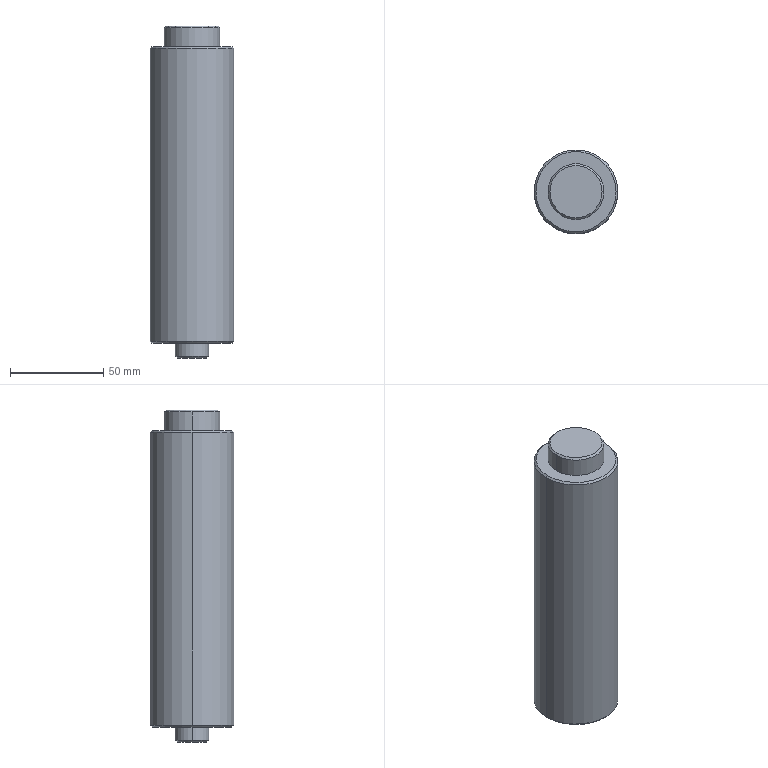Part | SolidWorks | features Chamfer 1, Revolution 1 | 1 solid | 18 faces | box 45 x 45 x 178 mm | volume 262477 mm3 | cone 8 | cylinder 6 | plane 4 | commonest cylinder face diameters 18 x2 30 x2 45 x2
STEP:
#1=CARTESIAN_POINT('',(-21.5,0.,-170.));
#2=VERTEX_POINT('',#1);
#3=CARTESIAN_POINT('',(21.5,0.,-170.));
#4=VERTEX_POINT('',#3);
#5=CARTESIAN_POINT('',(0.,0.,-170.));
#6=DIRECTION('',(0.,0.,-1.));
#7=DIRECTION('',(1.,0.,0.));
#8=AXIS2_PLACEMENT_3D('',#5,#6,#7);
#9=CIRCLE('',#8,21.5);
#10=EDGE_CURVE('',#2,#4,#9,.T.);
#11=ORIENTED_EDGE('',*,*,#10,.F.);
#12=CARTESIAN_POINT('',(-22.5,0.,-169.));
#13=VERTEX_POINT('',#12);
#14=CARTESIAN_POINT('',(-22.5,0.,-169.));
#15=DIRECTION('',(-0.7071,0.,0.7071));
#16=VECTOR('',#15,1000.);
#17=LINE('',#14,#16);
#18=EDGE_CURVE('',#2,#13,#17,.T.);
#19=ORIENTED_EDGE('',*,*,#18,.T.);
#20=CARTESIAN_POINT('',(22.5,0.,-169.));
#21=VERTEX_POINT('',#20);
#22=CARTESIAN_POINT('',(0.,0.,-169.));
#23=DIRECTION('',(0.,0.,1.));
#24=DIRECTION('',(1.,0.,0.));
#25=AXIS2_PLACEMENT_3D('',#22,#23,#24);
#26=CIRCLE('',#25,22.5);
#27=EDGE_CURVE('',#21,#13,#26,.T.);
#28=ORIENTED_EDGE('',*,*,#27,.F.);
#29=CARTESIAN_POINT('',(22.5,0.,-169.));
#30=DIRECTION('',(0.7071,0.,0.7071));
#31=VECTOR('',#30,1000.);
#32=LINE('',#29,#31);
#33=EDGE_CURVE('',#4,#21,#32,.T.);
#34=ORIENTED_EDGE('',*,*,#33,.F.);
#35=EDGE_LOOP('',(#11,#19,#28,#34));
#36=FACE_OUTER_BOUND('',#35,.T.);
#37=CARTESIAN_POINT('',(0.,0.,-169.));
#38=DIRECTION('',(0.,0.,1.));
#39=DIRECTION('',(1.,0.,0.));
#40=AXIS2_PLACEMENT_3D('',#37,#38,#39);
#41=CONICAL_SURFACE('',#40,22.5,0.7854);
#42=ADVANCED_FACE('',(#36),#41,.T.);
#43=CARTESIAN_POINT('',(-8.,0.,-178.));
#44=VERTEX_POINT('',#43);
#45=CARTESIAN_POINT('',(8.,0.,-178.));
#46=VERTEX_POINT('',#45);
#47=CARTESIAN_POINT('',(0.,0.,-178.));
#48=DIRECTION('',(0.,0.,-1.));
#49=DIRECTION('',(1.,0.,0.));
#50=AXIS2_PLACEMENT_3D('',#47,#48,#49);
#51=CIRCLE('',#50,8.);
#52=EDGE_CURVE('',#44,#46,#51,.T.);
#53=ORIENTED_EDGE('',*,*,#52,.F.);
#54=CARTESIAN_POINT('',(-9.,0.,-177.));
#55=VERTEX_POINT('',#54);
#56=CARTESIAN_POINT('',(-9.,0.,-177.));
#57=DIRECTION('',(-0.7071,0.,0.7071));
#58=VECTOR('',#57,1000.);
#59=LINE('',#56,#58);
#60=EDGE_CURVE('',#44,#55,#59,.T.);
#61=ORIENTED_EDGE('',*,*,#60,.T.);
#62=CARTESIAN_POINT('',(9.,0.,-177.));
#63=VERTEX_POINT('',#62);
#64=CARTESIAN_POINT('',(0.,0.,-177.));
#65=DIRECTION('',(0.,0.,1.));
#66=DIRECTION('',(1.,0.,0.));
#67=AXIS2_PLACEMENT_3D('',#64,#65,#66);
#68=CIRCLE('',#67,9.);
#69=EDGE_CURVE('',#63,#55,#68,.T.);
#70=ORIENTED_EDGE('',*,*,#69,.F.);
#71=CARTESIAN_POINT('',(9.,0.,-177.));
#72=DIRECTION('',(0.7071,0.,0.7071));
#73=VECTOR('',#72,1000.);
#74=LINE('',#71,#73);
#75=EDGE_CURVE('',#46,#63,#74,.T.);
#76=ORIENTED_EDGE('',*,*,#75,.F.);
#77=EDGE_LOOP('',(#53,#61,#70,#76));
#78=FACE_OUTER_BOUND('',#77,.T.);
#79=CARTESIAN_POINT('',(0.,0.,-177.));
#80=DIRECTION('',(0.,0.,1.));
#81=DIRECTION('',(1.,0.,0.));
#82=AXIS2_PLACEMENT_3D('',#79,#80,#81);
#83=CONICAL_SURFACE('',#82,9.,0.7854);
#84=ADVANCED_FACE('',(#78),#83,.T.);
#85=CARTESIAN_POINT('',(21.5,0.,-11.));
#86=VERTEX_POINT('',#85);
#87=CARTESIAN_POINT('',(-21.5,0.,-11.));
#88=VERTEX_POINT('',#87);
#89=CARTESIAN_POINT('',(0.,0.,-11.));
#90=DIRECTION('',(0.,0.,1.));
#91=DIRECTION('',(-1.,0.,0.));
#92=AXIS2_PLACEMENT_3D('',#89,#90,#91);
#93=CIRCLE('',#92,21.5);
#94=EDGE_CURVE('',#86,#88,#93,.T.);
#95=ORIENTED_EDGE('',*,*,#94,.F.);
#96=CARTESIAN_POINT('',(22.5,0.,-12.));
#97=VERTEX_POINT('',#96);
#98=CARTESIAN_POINT('',(21.5,0.,-11.));
#99=DIRECTION('',(0.7071,0.,-0.7071));
#100=VECTOR('',#99,1000.);
#101=LINE('',#98,#100);
#102=EDGE_CURVE('',#86,#97,#101,.T.);
#103=ORIENTED_EDGE('',*,*,#102,.T.);
#104=CARTESIAN_POINT('',(-22.5,0.,-12.));
#105=VERTEX_POINT('',#104);
#106=CARTESIAN_POINT('',(0.,0.,-12.));
#107=DIRECTION('',(0.,0.,-1.));
#108=DIRECTION('',(-1.,0.,0.));
#109=AXIS2_PLACEMENT_3D('',#106,#107,#108);
#110=CIRCLE('',#109,22.5);
#111=EDGE_CURVE('',#105,#97,#110,.T.);
#112=ORIENTED_EDGE('',*,*,#111,.F.);
#113=CARTESIAN_POINT('',(-21.5,0.,-11.));
#114=DIRECTION('',(-0.7071,0.,-0.7071));
#115=VECTOR('',#114,1000.);
#116=LINE('',#113,#115);
#117=EDGE_CURVE('',#88,#105,#116,.T.);
#118=ORIENTED_EDGE('',*,*,#117,.F.);
#119=EDGE_LOOP('',(#95,#103,#112,#118));
#120=FACE_OUTER_BOUND('',#119,.T.);
#121=CARTESIAN_POINT('',(0.,0.,-11.));
#122=DIRECTION('',(0.,0.,-1.));
#123=DIRECTION('',(-1.,0.,0.));
#124=AXIS2_PLACEMENT_3D('',#121,#122,#123);
#125=CONICAL_SURFACE('',#124,21.5,0.7854);
#126=ADVANCED_FACE('',(#120),#125,.T.);
#127=CARTESIAN_POINT('',(14.,0.,0.));
#128=VERTEX_POINT('',#127);
#129=CARTESIAN_POINT('',(-14.,0.,0.));
#130=VERTEX_POINT('',#129);
#131=CARTESIAN_POINT('',(0.,0.,0.));
#132=DIRECTION('',(0.,0.,1.));
#133=DIRECTION('',(-1.,0.,0.));
#134=AXIS2_PLACEMENT_3D('',#131,#132,#133);
#135=CIRCLE('',#134,14.);
#136=EDGE_CURVE('',#128,#130,#135,.T.);
#137=ORIENTED_EDGE('',*,*,#136,.F.);
#138=CARTESIAN_POINT('',(15.,0.,-1.));
#139=VERTEX_POINT('',#138);
#140=CARTESIAN_POINT('',(14.,0.,0.));
#141=DIRECTION('',(0.7071,0.,-0.7071));
#142=VECTOR('',#141,1000.);
#143=LINE('',#140,#142);
#144=EDGE_CURVE('',#128,#139,#143,.T.);
#145=ORIENTED_EDGE('',*,*,#144,.T.);
#146=CARTESIAN_POINT('',(-15.,0.,-1.));
#147=VERTEX_POINT('',#146);
#148=CARTESIAN_POINT('',(0.,0.,-1.));
#149=DIRECTION('',(0.,0.,-1.));
#150=DIRECTION('',(-1.,0.,0.));
#151=AXIS2_PLACEMENT_3D('',#148,#149,#150);
#152=CIRCLE('',#151,15.);
#153=EDGE_CURVE('',#147,#139,#152,.T.);
#154=ORIENTED_EDGE('',*,*,#153,.F.);
#155=CARTESIAN_POINT('',(-14.,0.,0.));
#156=DIRECTION('',(-0.7071,0.,-0.7071));
#157=VECTOR('',#156,1000.);
#158=LINE('',#155,#157);
#159=EDGE_CURVE('',#130,#147,#158,.T.);
#160=ORIENTED_EDGE('',*,*,#159,.F.);
#161=EDGE_LOOP('',(#137,#145,#154,#160));
#162=FACE_OUTER_BOUND('',#161,.T.);
#163=CARTESIAN_POINT('',(0.,0.,0.));
#164=DIRECTION('',(0.,0.,-1.));
#165=DIRECTION('',(-1.,0.,0.));
#166=AXIS2_PLACEMENT_3D('',#163,#164,#165);
#167=CONICAL_SURFACE('',#166,14.,0.7854);
#168=ADVANCED_FACE('',(#162),#167,.T.);
#169=CARTESIAN_POINT('',(15.,0.,-11.));
#170=VERTEX_POINT('',#169);
#171=CARTESIAN_POINT('',(-15.,0.,-11.));
#172=VERTEX_POINT('',#171);
#173=CARTESIAN_POINT('',(0.,0.,-11.));
#174=DIRECTION('',(0.,0.,1.));
#175=DIRECTION('',(1.,0.,0.));
#176=AXIS2_PLACEMENT_3D('',#173,#174,#175);
#177=CIRCLE('',#176,15.);
#178=EDGE_CURVE('',#170,#172,#177,.T.);
#179=ORIENTED_EDGE('',*,*,#178,.T.);
#180=CARTESIAN_POINT('',(-15.,0.,0.));
#181=DIRECTION('',(0.,0.,1.));
#182=VECTOR('',#181,1000.);
#183=LINE('',#180,#182);
#184=EDGE_CURVE('',#172,#147,#183,.T.);
#185=ORIENTED_EDGE('',*,*,#184,.T.);
#186=ORIENTED_EDGE('',*,*,#153,.T.);
#187=CARTESIAN_POINT('',(15.,0.,0.));
#188=DIRECTION('',(0.,0.,1.));
#189=VECTOR('',#188,1000.);
#190=LINE('',#187,#189);
#191=EDGE_CURVE('',#170,#139,#190,.T.);
#192=ORIENTED_EDGE('',*,*,#191,.F.);
#193=EDGE_LOOP('',(#179,#185,#186,#192));
#194=FACE_OUTER_BOUND('',#193,.T.);
#195=CARTESIAN_POINT('',(0.,0.,0.));
#196=DIRECTION('',(0.,0.,1.));
#197=DIRECTION('',(1.,0.,0.));
#198=AXIS2_PLACEMENT_3D('',#195,#196,#197);
#199=CYLINDRICAL_SURFACE('',#198,15.);
#200=ADVANCED_FACE('',(#194),#199,.T.);
#201=ORIENTED_EDGE('',*,*,#27,.T.);
#202=CARTESIAN_POINT('',(-22.5,0.,0.));
#203=DIRECTION('',(0.,0.,1.));
#204=VECTOR('',#203,1000.);
#205=LINE('',#202,#204);
#206=EDGE_CURVE('',#13,#105,#205,.T.);
#207=ORIENTED_EDGE('',*,*,#206,.T.);
#208=ORIENTED_EDGE('',*,*,#111,.T.);
#209=CARTESIAN_POINT('',(22.5,0.,0.));
#210=DIRECTION('',(0.,0.,1.));
#211=VECTOR('',#210,1000.);
#212=LINE('',#209,#211);
#213=EDGE_CURVE('',#21,#97,#212,.T.);
#214=ORIENTED_EDGE('',*,*,#213,.F.);
#215=EDGE_LOOP('',(#201,#207,#208,#214));
#216=FACE_OUTER_BOUND('',#215,.T.);
#217=CARTESIAN_POINT('',(0.,0.,0.));
#218=DIRECTION('',(0.,0.,1.));
#219=DIRECTION('',(1.,0.,0.));
#220=AXIS2_PLACEMENT_3D('',#217,#218,#219);
#221=CYLINDRICAL_SURFACE('',#220,22.5);
#222=ADVANCED_FACE('',(#216),#221,.T.);
#223=ORIENTED_EDGE('',*,*,#69,.T.);
#224=CARTESIAN_POINT('',(-9.,0.,-170.));
#225=VERTEX_POINT('',#224);
#226=CARTESIAN_POINT('',(-9.,0.,0.));
#227=DIRECTION('',(0.,0.,1.));
#228=VECTOR('',#227,1000.);
#229=LINE('',#226,#228);
#230=EDGE_CURVE('',#55,#225,#229,.T.);
#231=ORIENTED_EDGE('',*,*,#230,.T.);
#232=CARTESIAN_POINT('',(9.,0.,-170.));
#233=VERTEX_POINT('',#232);
#234=CARTESIAN_POINT('',(0.,0.,-170.));
#235=DIRECTION('',(0.,0.,1.));
#236=DIRECTION('',(1.,0.,0.));
#237=AXIS2_PLACEMENT_3D('',#234,#235,#236);
#238=CIRCLE('',#237,9.);
#239=EDGE_CURVE('',#233,#225,#238,.T.);
#240=ORIENTED_EDGE('',*,*,#239,.F.);
#241=CARTESIAN_POINT('',(9.,0.,0.));
#242=DIRECTION('',(0.,0.,1.));
#243=VECTOR('',#242,1000.);
#244=LINE('',#241,#243);
#245=EDGE_CURVE('',#63,#233,#244,.T.);
#246=ORIENTED_EDGE('',*,*,#245,.F.);
#247=EDGE_LOOP('',(#223,#231,#240,#246));
#248=FACE_OUTER_BOUND('',#247,.T.);
#249=CARTESIAN_POINT('',(0.,0.,0.));
#250=DIRECTION('',(0.,0.,1.));
#251=DIRECTION('',(1.,0.,0.));
#252=AXIS2_PLACEMENT_3D('',#249,#250,#251);
#253=CYLINDRICAL_SURFACE('',#252,9.);
#254=ADVANCED_FACE('',(#248),#253,.T.);
#255=CARTESIAN_POINT('',(0.,0.,-178.));
#256=DIRECTION('',(0.,0.,-1.));
#257=DIRECTION('',(1.,0.,0.));
#258=AXIS2_PLACEMENT_3D('',#255,#256,#257);
#259=CIRCLE('',#258,8.);
#260=EDGE_CURVE('',#46,#44,#259,.T.);
#261=ORIENTED_EDGE('',*,*,#260,.T.);
#262=ORIENTED_EDGE('',*,*,#52,.T.);
#263=EDGE_LOOP('',(#261,#262));
#264=FACE_OUTER_BOUND('',#263,.T.);
#265=CARTESIAN_POINT('',(0.,0.,-178.));
#266=DIRECTION('',(0.,0.,1.));
#267=DIRECTION('',(1.,0.,0.));
#268=AXIS2_PLACEMENT_3D('',#265,#266,#267);
#269=PLANE('',#268);
#270=ADVANCED_FACE('',(#264),#269,.F.);
#271=ORIENTED_EDGE('',*,*,#230,.F.);
#272=CARTESIAN_POINT('',(0.,0.,-177.));
#273=DIRECTION('',(0.,0.,1.));
#274=DIRECTION('',(1.,0.,0.));
#275=AXIS2_PLACEMENT_3D('',#272,#273,#274);
#276=CIRCLE('',#275,9.);
#277=EDGE_CURVE('',#55,#63,#276,.T.);
#278=ORIENTED_EDGE('',*,*,#277,.T.);
#279=ORIENTED_EDGE('',*,*,#245,.T.);
#280=CARTESIAN_POINT('',(0.,0.,-170.));
#281=DIRECTION('',(0.,0.,1.));
#282=DIRECTION('',(1.,0.,0.));
#283=AXIS2_PLACEMENT_3D('',#280,#281,#282);
#284=CIRCLE('',#283,9.);
#285=EDGE_CURVE('',#225,#233,#284,.T.);
#286=ORIENTED_EDGE('',*,*,#285,.F.);
#287=EDGE_LOOP('',(#271,#278,#279,#286));
#288=FACE_OUTER_BOUND('',#287,.T.);
#289=CARTESIAN_POINT('',(0.,0.,0.));
#290=DIRECTION('',(0.,0.,1.));
#291=DIRECTION('',(1.,0.,0.));
#292=AXIS2_PLACEMENT_3D('',#289,#290,#291);
#293=CYLINDRICAL_SURFACE('',#292,9.);
#294=ADVANCED_FACE('',(#288),#293,.T.);
#295=CARTESIAN_POINT('',(0.,0.,-170.));
#296=DIRECTION('',(0.,0.,-1.));
#297=DIRECTION('',(1.,0.,0.));
#298=AXIS2_PLACEMENT_3D('',#295,#296,#297);
#299=CIRCLE('',#298,21.5);
#300=EDGE_CURVE('',#4,#2,#299,.T.);
#301=ORIENTED_EDGE('',*,*,#300,.T.);
#302=ORIENTED_EDGE('',*,*,#10,.T.);
#303=EDGE_LOOP('',(#301,#302));
#304=FACE_OUTER_BOUND('',#303,.T.);
#305=ORIENTED_EDGE('',*,*,#239,.T.);
#306=ORIENTED_EDGE('',*,*,#285,.T.);
#307=EDGE_LOOP('',(#305,#306));
#308=FACE_BOUND('',#307,.T.);
#309=CARTESIAN_POINT('',(0.,9.,-170.));
#310=DIRECTION('',(0.,0.,1.));
#311=DIRECTION('',(1.,0.,0.));
#312=AXIS2_PLACEMENT_3D('',#309,#310,#311);
#313=PLANE('',#312);
#314=ADVANCED_FACE('',(#304,#308),#313,.F.);
#315=ORIENTED_EDGE('',*,*,#206,.F.);
#316=CARTESIAN_POINT('',(0.,0.,-169.));
#317=DIRECTION('',(0.,0.,1.));
#318=DIRECTION('',(1.,0.,0.));
#319=AXIS2_PLACEMENT_3D('',#316,#317,#318);
#320=CIRCLE('',#319,22.5);
#321=EDGE_CURVE('',#13,#21,#320,.T.);
#322=ORIENTED_EDGE('',*,*,#321,.T.);
#323=ORIENTED_EDGE('',*,*,#213,.T.);
#324=CARTESIAN_POINT('',(0.,0.,-12.));
#325=DIRECTION('',(0.,0.,-1.));
#326=DIRECTION('',(-1.,0.,0.));
#327=AXIS2_PLACEMENT_3D('',#324,#325,#326);
#328=CIRCLE('',#327,22.5);
#329=EDGE_CURVE('',#97,#105,#328,.T.);
#330=ORIENTED_EDGE('',*,*,#329,.T.);
#331=EDGE_LOOP('',(#315,#322,#323,#330));
#332=FACE_OUTER_BOUND('',#331,.T.);
#333=CARTESIAN_POINT('',(0.,0.,0.));
#334=DIRECTION('',(0.,0.,1.));
#335=DIRECTION('',(1.,0.,0.));
#336=AXIS2_PLACEMENT_3D('',#333,#334,#335);
#337=CYLINDRICAL_SURFACE('',#336,22.5);
#338=ADVANCED_FACE('',(#332),#337,.T.);
#339=CARTESIAN_POINT('',(0.,0.,-11.));
#340=DIRECTION('',(0.,0.,1.));
#341=DIRECTION('',(-1.,0.,0.));
#342=AXIS2_PLACEMENT_3D('',#339,#340,#341);
#343=CIRCLE('',#342,21.5);
#344=EDGE_CURVE('',#88,#86,#343,.T.);
#345=ORIENTED_EDGE('',*,*,#344,.T.);
#346=ORIENTED_EDGE('',*,*,#94,.T.);
#347=EDGE_LOOP('',(#345,#346));
#348=FACE_OUTER_BOUND('',#347,.T.);
#349=ORIENTED_EDGE('',*,*,#178,.F.);
#350=CARTESIAN_POINT('',(0.,0.,-11.));
#351=DIRECTION('',(0.,0.,1.));
#352=DIRECTION('',(1.,0.,0.));
#353=AXIS2_PLACEMENT_3D('',#350,#351,#352);
#354=CIRCLE('',#353,15.);
#355=EDGE_CURVE('',#172,#170,#354,.T.);
#356=ORIENTED_EDGE('',*,*,#355,.F.);
#357=EDGE_LOOP('',(#349,#356));
#358=FACE_BOUND('',#357,.T.);
#359=CARTESIAN_POINT('',(0.,22.5,-11.));
#360=DIRECTION('',(0.,0.,-1.));
#361=DIRECTION('',(-1.,0.,0.));
#362=AXIS2_PLACEMENT_3D('',#359,#360,#361);
#363=PLANE('',#362);
#364=ADVANCED_FACE('',(#348,#358),#363,.F.);
#365=ORIENTED_EDGE('',*,*,#184,.F.);
#366=ORIENTED_EDGE('',*,*,#355,.T.);
#367=ORIENTED_EDGE('',*,*,#191,.T.);
#368=CARTESIAN_POINT('',(0.,0.,-1.));
#369=DIRECTION('',(0.,0.,-1.));
#370=DIRECTION('',(-1.,0.,0.));
#371=AXIS2_PLACEMENT_3D('',#368,#369,#370);
#372=CIRCLE('',#371,15.);
#373=EDGE_CURVE('',#139,#147,#372,.T.);
#374=ORIENTED_EDGE('',*,*,#373,.T.);
#375=EDGE_LOOP('',(#365,#366,#367,#374));
#376=FACE_OUTER_BOUND('',#375,.T.);
#377=CARTESIAN_POINT('',(0.,0.,0.));
#378=DIRECTION('',(0.,0.,1.));
#379=DIRECTION('',(1.,0.,0.));
#380=AXIS2_PLACEMENT_3D('',#377,#378,#379);
#381=CYLINDRICAL_SURFACE('',#380,15.);
#382=ADVANCED_FACE('',(#376),#381,.T.);
#383=CARTESIAN_POINT('',(0.,0.,0.));
#384=DIRECTION('',(0.,0.,1.));
#385=DIRECTION('',(-1.,0.,0.));
#386=AXIS2_PLACEMENT_3D('',#383,#384,#385);
#387=CIRCLE('',#386,14.);
#388=EDGE_CURVE('',#130,#128,#387,.T.);
#389=ORIENTED_EDGE('',*,*,#388,.T.);
#390=ORIENTED_EDGE('',*,*,#136,.T.);
#391=EDGE_LOOP('',(#389,#390));
#392=FACE_OUTER_BOUND('',#391,.T.);
#393=CARTESIAN_POINT('',(0.,15.,0.));
#394=DIRECTION('',(0.,0.,-1.));
#395=DIRECTION('',(-1.,0.,0.));
#396=AXIS2_PLACEMENT_3D('',#393,#394,#395);
#397=PLANE('',#396);
#398=ADVANCED_FACE('',(#392),#397,.F.);
#399=ORIENTED_EDGE('',*,*,#144,.F.);
#400=ORIENTED_EDGE('',*,*,#388,.F.);
#401=ORIENTED_EDGE('',*,*,#159,.T.);
#402=ORIENTED_EDGE('',*,*,#373,.F.);
#403=EDGE_LOOP('',(#399,#400,#401,#402));
#404=FACE_OUTER_BOUND('',#403,.T.);
#405=CARTESIAN_POINT('',(0.,0.,0.));
#406=DIRECTION('',(0.,0.,-1.));
#407=DIRECTION('',(-1.,0.,0.));
#408=AXIS2_PLACEMENT_3D('',#405,#406,#407);
#409=CONICAL_SURFACE('',#408,14.,0.7854);
#410=ADVANCED_FACE('',(#404),#409,.T.);
#411=ORIENTED_EDGE('',*,*,#102,.F.);
#412=ORIENTED_EDGE('',*,*,#344,.F.);
#413=ORIENTED_EDGE('',*,*,#117,.T.);
#414=ORIENTED_EDGE('',*,*,#329,.F.);
#415=EDGE_LOOP('',(#411,#412,#413,#414));
#416=FACE_OUTER_BOUND('',#415,.T.);
#417=CARTESIAN_POINT('',(0.,0.,-11.));
#418=DIRECTION('',(0.,0.,-1.));
#419=DIRECTION('',(-1.,0.,0.));
#420=AXIS2_PLACEMENT_3D('',#417,#418,#419);
#421=CONICAL_SURFACE('',#420,21.5,0.7854);
#422=ADVANCED_FACE('',(#416),#421,.T.);
#423=ORIENTED_EDGE('',*,*,#60,.F.);
#424=ORIENTED_EDGE('',*,*,#260,.F.);
#425=ORIENTED_EDGE('',*,*,#75,.T.);
#426=ORIENTED_EDGE('',*,*,#277,.F.);
#427=EDGE_LOOP('',(#423,#424,#425,#426));
#428=FACE_OUTER_BOUND('',#427,.T.);
#429=CARTESIAN_POINT('',(0.,0.,-177.));
#430=DIRECTION('',(0.,0.,1.));
#431=DIRECTION('',(1.,0.,0.));
#432=AXIS2_PLACEMENT_3D('',#429,#430,#431);
#433=CONICAL_SURFACE('',#432,9.,0.7854);
#434=ADVANCED_FACE('',(#428),#433,.T.);
#435=ORIENTED_EDGE('',*,*,#18,.F.);
#436=ORIENTED_EDGE('',*,*,#300,.F.);
#437=ORIENTED_EDGE('',*,*,#33,.T.);
#438=ORIENTED_EDGE('',*,*,#321,.F.);
#439=EDGE_LOOP('',(#435,#436,#437,#438));
#440=FACE_OUTER_BOUND('',#439,.T.);
#441=CARTESIAN_POINT('',(0.,0.,-169.));
#442=DIRECTION('',(0.,0.,1.));
#443=DIRECTION('',(1.,0.,0.));
#444=AXIS2_PLACEMENT_3D('',#441,#442,#443);
#445=CONICAL_SURFACE('',#444,22.5,0.7854);
#446=ADVANCED_FACE('',(#440),#445,.T.);
#447=CLOSED_SHELL('',(#42,#84,#126,#168,#200,#222,#254,#270,#294,#314,#338,#364,#382,#398,#410,#422,#434,#446));
#448=MANIFOLD_SOLID_BREP('',#447);
#449=CARTESIAN_POINT('',(0.,0.,0.));
#450=DIRECTION('',(0.,0.,1.));
#451=DIRECTION('',(1.,0.,0.));
#452=AXIS2_PLACEMENT_3D('',#449,#450,#451);
#453=(LENGTH_UNIT()NAMED_UNIT(*)SI_UNIT(.MILLI.,.METRE.));
#454=UNCERTAINTY_MEASURE_WITH_UNIT(LENGTH_MEASURE(0.00001),#453,'','');
#455=(NAMED_UNIT(*)PLANE_ANGLE_UNIT()SI_UNIT($,.RADIAN.));
#456=(NAMED_UNIT(*)SI_UNIT($,.STERADIAN.)SOLID_ANGLE_UNIT());
#457=(GEOMETRIC_REPRESENTATION_CONTEXT(3)GLOBAL_UNCERTAINTY_ASSIGNED_CONTEXT((#454))GLOBAL_UNIT_ASSIGNED_CONTEXT((#453,#455,#456))REPRESENTATION_CONTEXT('',''));
#458=ADVANCED_BREP_SHAPE_REPRESENTATION('',(#448,#452),#457);